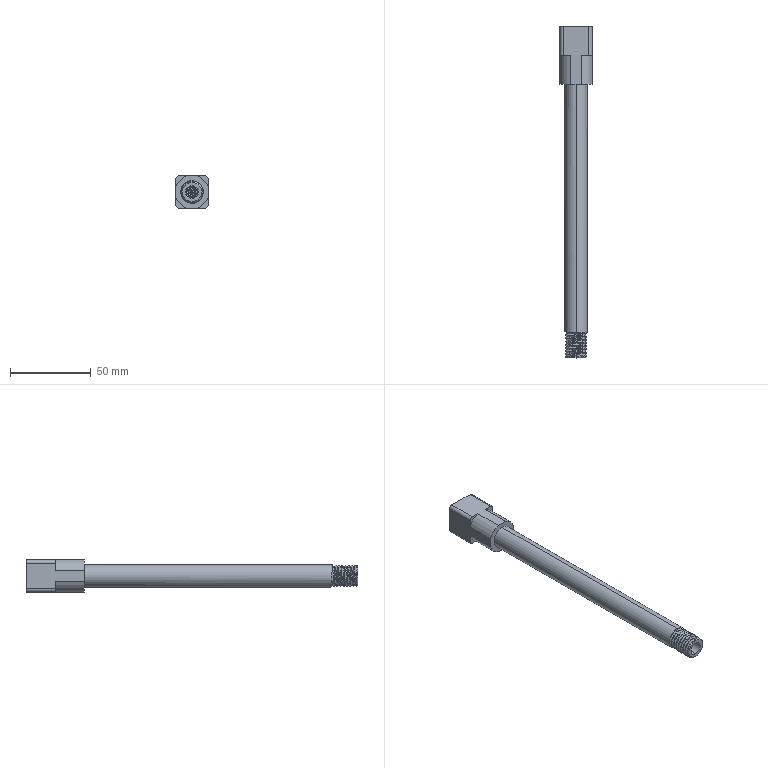Part | SolidWorks | features BaseBody 1 | 1 solid | 116 faces | box 20 x 206 x 20 mm | volume 27398 mm3 | cylinder 83 | plane 16 | spline 11 | cone 6 | commonest cylinder face diameters 13.6 x36 11.6 x35 4 x4 21 x4 8 x2 14 x2